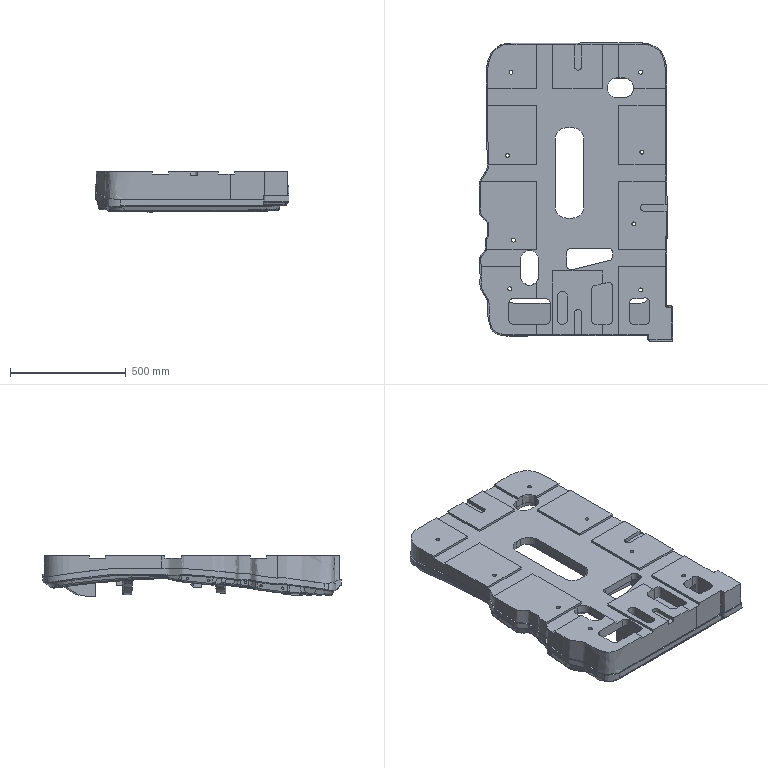Part | NX | features solid 2 | 1 solid | 797 faces | box 835.512 x 1287 x 175.683 mm | volume 74930313 mm3 | spline 532 | plane 194 | cylinder 67 | cone 4 | commonest cylinder face diameters 40 x20 25 x16 32 x9 17 x8 16 x4 60 x4